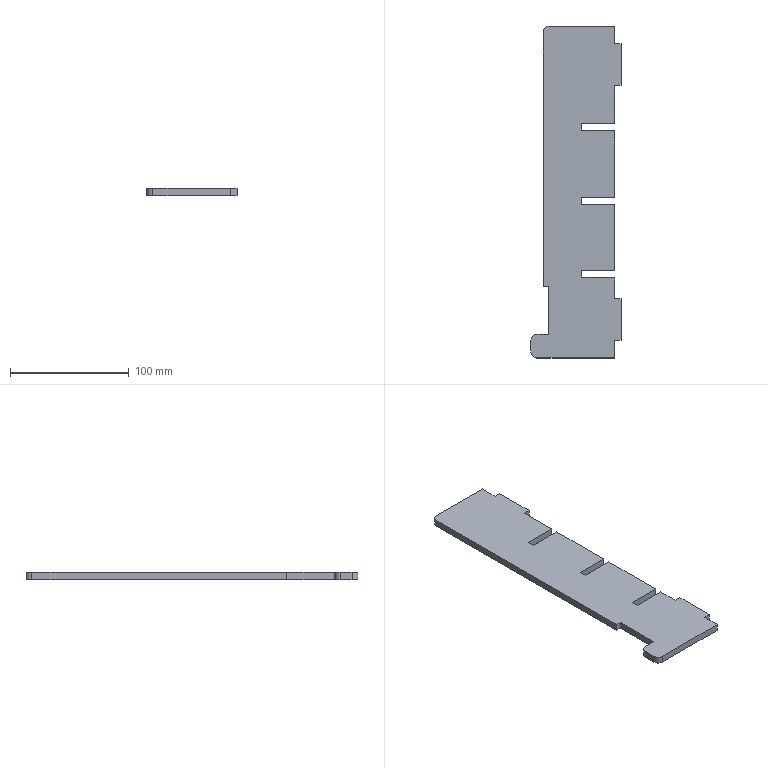Part | SolidWorks | features Fillet 1, FlatPattern 1, SMBaseFlange 1, SheetMetal 1 | 1 solid | 33 faces | box 76 x 280 x 6 mm | volume 100169 mm3 | plane 30 | cylinder 3 | commonest cylinder face diameters 10 x3
STEP:
#1=CARTESIAN_POINT('',(-245.,-135.834,0.));
#2=VERTEX_POINT('',#1);
#3=CARTESIAN_POINT('',(-255.,-135.834,0.));
#4=VERTEX_POINT('',#3);
#5=CARTESIAN_POINT('',(-245.,-135.834,0.));
#6=DIRECTION('',(-1.,0.,0.));
#7=VECTOR('',#6,1000.);
#8=LINE('',#5,#7);
#9=EDGE_CURVE('',#2,#4,#8,.T.);
#10=ORIENTED_EDGE('',*,*,#9,.T.);
#11=CARTESIAN_POINT('',(-255.,-135.834,6.));
#12=VERTEX_POINT('',#11);
#13=CARTESIAN_POINT('',(-255.,-135.834,6.));
#14=DIRECTION('',(0.,0.,1.));
#15=VECTOR('',#14,1000.);
#16=LINE('',#13,#15);
#17=EDGE_CURVE('',#4,#12,#16,.T.);
#18=ORIENTED_EDGE('',*,*,#17,.T.);
#19=CARTESIAN_POINT('',(-245.,-135.834,6.));
#20=VERTEX_POINT('',#19);
#21=CARTESIAN_POINT('',(-245.,-135.834,6.));
#22=DIRECTION('',(-1.,0.,0.));
#23=VECTOR('',#22,1000.);
#24=LINE('',#21,#23);
#25=EDGE_CURVE('',#20,#12,#24,.T.);
#26=ORIENTED_EDGE('',*,*,#25,.F.);
#27=CARTESIAN_POINT('',(-245.,-135.834,6.));
#28=DIRECTION('',(0.,0.,-1.));
#29=VECTOR('',#28,1000.);
#30=LINE('',#27,#29);
#31=EDGE_CURVE('',#20,#2,#30,.T.);
#32=ORIENTED_EDGE('',*,*,#31,.T.);
#33=EDGE_LOOP('',(#10,#18,#26,#32));
#34=FACE_OUTER_BOUND('',#33,.T.);
#35=CARTESIAN_POINT('',(-245.,-135.834,6.));
#36=DIRECTION('',(0.,-1.,0.));
#37=DIRECTION('',(0.,0.,-1.));
#38=AXIS2_PLACEMENT_3D('',#35,#36,#37);
#39=PLANE('',#38);
#40=ADVANCED_FACE('',(#34),#39,.F.);
#41=CARTESIAN_POINT('',(-260.,-140.834,6.));
#42=VERTEX_POINT('',#41);
#43=CARTESIAN_POINT('',(-260.,-150.834,6.));
#44=VERTEX_POINT('',#43);
#45=CARTESIAN_POINT('',(-260.,-135.834,6.));
#46=DIRECTION('',(0.,-1.,0.));
#47=VECTOR('',#46,1000.);
#48=LINE('',#45,#47);
#49=EDGE_CURVE('',#42,#44,#48,.T.);
#50=ORIENTED_EDGE('',*,*,#49,.F.);
#51=CARTESIAN_POINT('',(-260.,-140.834,0.));
#52=VERTEX_POINT('',#51);
#53=CARTESIAN_POINT('',(-260.,-140.834,6.));
#54=DIRECTION('',(0.,0.,-1.));
#55=VECTOR('',#54,1000.);
#56=LINE('',#53,#55);
#57=EDGE_CURVE('',#42,#52,#56,.T.);
#58=ORIENTED_EDGE('',*,*,#57,.T.);
#59=CARTESIAN_POINT('',(-260.,-150.834,0.));
#60=VERTEX_POINT('',#59);
#61=CARTESIAN_POINT('',(-260.,-135.834,0.));
#62=DIRECTION('',(0.,-1.,0.));
#63=VECTOR('',#62,1000.);
#64=LINE('',#61,#63);
#65=EDGE_CURVE('',#52,#60,#64,.T.);
#66=ORIENTED_EDGE('',*,*,#65,.T.);
#67=CARTESIAN_POINT('',(-260.,-150.834,6.));
#68=DIRECTION('',(0.,0.,1.));
#69=VECTOR('',#68,1000.);
#70=LINE('',#67,#69);
#71=EDGE_CURVE('',#60,#44,#70,.T.);
#72=ORIENTED_EDGE('',*,*,#71,.T.);
#73=EDGE_LOOP('',(#50,#58,#66,#72));
#74=FACE_OUTER_BOUND('',#73,.T.);
#75=CARTESIAN_POINT('',(-260.,-135.834,6.));
#76=DIRECTION('',(1.,0.,0.));
#77=DIRECTION('',(0.,0.,-1.));
#78=AXIS2_PLACEMENT_3D('',#75,#76,#77);
#79=PLANE('',#78);
#80=ADVANCED_FACE('',(#74),#79,.F.);
#81=CARTESIAN_POINT('',(-255.,-155.834,6.));
#82=VERTEX_POINT('',#81);
#83=CARTESIAN_POINT('',(-189.5,-155.834,6.));
#84=VERTEX_POINT('',#83);
#85=CARTESIAN_POINT('',(-260.,-155.834,6.));
#86=DIRECTION('',(1.,0.,0.));
#87=VECTOR('',#86,1000.);
#88=LINE('',#85,#87);
#89=EDGE_CURVE('',#82,#84,#88,.T.);
#90=ORIENTED_EDGE('',*,*,#89,.F.);
#91=CARTESIAN_POINT('',(-255.,-155.834,0.));
#92=VERTEX_POINT('',#91);
#93=CARTESIAN_POINT('',(-255.,-155.834,6.));
#94=DIRECTION('',(0.,0.,-1.));
#95=VECTOR('',#94,1000.);
#96=LINE('',#93,#95);
#97=EDGE_CURVE('',#82,#92,#96,.T.);
#98=ORIENTED_EDGE('',*,*,#97,.T.);
#99=CARTESIAN_POINT('',(-189.5,-155.834,0.));
#100=VERTEX_POINT('',#99);
#101=CARTESIAN_POINT('',(-260.,-155.834,0.));
#102=DIRECTION('',(1.,0.,0.));
#103=VECTOR('',#102,1000.);
#104=LINE('',#101,#103);
#105=EDGE_CURVE('',#92,#100,#104,.T.);
#106=ORIENTED_EDGE('',*,*,#105,.T.);
#107=CARTESIAN_POINT('',(-189.5,-155.834,6.));
#108=DIRECTION('',(0.,0.,-1.));
#109=VECTOR('',#108,1000.);
#110=LINE('',#107,#109);
#111=EDGE_CURVE('',#84,#100,#110,.T.);
#112=ORIENTED_EDGE('',*,*,#111,.F.);
#113=EDGE_LOOP('',(#90,#98,#106,#112));
#114=FACE_OUTER_BOUND('',#113,.T.);
#115=CARTESIAN_POINT('',(-260.,-155.834,6.));
#116=DIRECTION('',(0.,1.,0.));
#117=DIRECTION('',(0.,0.,1.));
#118=AXIS2_PLACEMENT_3D('',#115,#116,#117);
#119=PLANE('',#118);
#120=ADVANCED_FACE('',(#114),#119,.F.);
#121=CARTESIAN_POINT('',(-189.5,-140.834,0.));
#122=VERTEX_POINT('',#121);
#123=CARTESIAN_POINT('',(-189.5,-155.834,0.));
#124=DIRECTION('',(0.,1.,0.));
#125=VECTOR('',#124,1000.);
#126=LINE('',#123,#125);
#127=EDGE_CURVE('',#100,#122,#126,.T.);
#128=ORIENTED_EDGE('',*,*,#127,.T.);
#129=CARTESIAN_POINT('',(-189.5,-140.834,6.));
#130=VERTEX_POINT('',#129);
#131=CARTESIAN_POINT('',(-189.5,-140.834,6.));
#132=DIRECTION('',(0.,0.,-1.));
#133=VECTOR('',#132,1000.);
#134=LINE('',#131,#133);
#135=EDGE_CURVE('',#130,#122,#134,.T.);
#136=ORIENTED_EDGE('',*,*,#135,.F.);
#137=CARTESIAN_POINT('',(-189.5,-155.834,6.));
#138=DIRECTION('',(0.,1.,0.));
#139=VECTOR('',#138,1000.);
#140=LINE('',#137,#139);
#141=EDGE_CURVE('',#84,#130,#140,.T.);
#142=ORIENTED_EDGE('',*,*,#141,.F.);
#143=ORIENTED_EDGE('',*,*,#111,.T.);
#144=EDGE_LOOP('',(#128,#136,#142,#143));
#145=FACE_OUTER_BOUND('',#144,.T.);
#146=CARTESIAN_POINT('',(-189.5,-155.834,6.));
#147=DIRECTION('',(-1.,0.,0.));
#148=DIRECTION('',(0.,-1.,0.));
#149=AXIS2_PLACEMENT_3D('',#146,#147,#148);
#150=PLANE('',#149);
#151=ADVANCED_FACE('',(#145),#150,.F.);
#152=CARTESIAN_POINT('',(-184.,-140.834,0.));
#153=VERTEX_POINT('',#152);
#154=CARTESIAN_POINT('',(-189.5,-140.834,0.));
#155=DIRECTION('',(1.,0.,0.));
#156=VECTOR('',#155,1000.);
#157=LINE('',#154,#156);
#158=EDGE_CURVE('',#122,#153,#157,.T.);
#159=ORIENTED_EDGE('',*,*,#158,.T.);
#160=CARTESIAN_POINT('',(-184.,-140.834,6.));
#161=VERTEX_POINT('',#160);
#162=CARTESIAN_POINT('',(-184.,-140.834,6.));
#163=DIRECTION('',(0.,0.,-1.));
#164=VECTOR('',#163,1000.);
#165=LINE('',#162,#164);
#166=EDGE_CURVE('',#161,#153,#165,.T.);
#167=ORIENTED_EDGE('',*,*,#166,.F.);
#168=CARTESIAN_POINT('',(-189.5,-140.834,6.));
#169=DIRECTION('',(1.,0.,0.));
#170=VECTOR('',#169,1000.);
#171=LINE('',#168,#170);
#172=EDGE_CURVE('',#130,#161,#171,.T.);
#173=ORIENTED_EDGE('',*,*,#172,.F.);
#174=ORIENTED_EDGE('',*,*,#135,.T.);
#175=EDGE_LOOP('',(#159,#167,#173,#174));
#176=FACE_OUTER_BOUND('',#175,.T.);
#177=CARTESIAN_POINT('',(-189.5,-140.834,6.));
#178=DIRECTION('',(0.,1.,0.));
#179=DIRECTION('',(0.,0.,1.));
#180=AXIS2_PLACEMENT_3D('',#177,#178,#179);
#181=PLANE('',#180);
#182=ADVANCED_FACE('',(#176),#181,.F.);
#183=CARTESIAN_POINT('',(-184.,-105.834,0.));
#184=VERTEX_POINT('',#183);
#185=CARTESIAN_POINT('',(-184.,-140.834,0.));
#186=DIRECTION('',(0.,1.,0.));
#187=VECTOR('',#186,1000.);
#188=LINE('',#185,#187);
#189=EDGE_CURVE('',#153,#184,#188,.T.);
#190=ORIENTED_EDGE('',*,*,#189,.T.);
#191=CARTESIAN_POINT('',(-184.,-105.834,6.));
#192=VERTEX_POINT('',#191);
#193=CARTESIAN_POINT('',(-184.,-105.834,6.));
#194=DIRECTION('',(0.,0.,-1.));
#195=VECTOR('',#194,1000.);
#196=LINE('',#193,#195);
#197=EDGE_CURVE('',#192,#184,#196,.T.);
#198=ORIENTED_EDGE('',*,*,#197,.F.);
#199=CARTESIAN_POINT('',(-184.,-140.834,6.));
#200=DIRECTION('',(0.,1.,0.));
#201=VECTOR('',#200,1000.);
#202=LINE('',#199,#201);
#203=EDGE_CURVE('',#161,#192,#202,.T.);
#204=ORIENTED_EDGE('',*,*,#203,.F.);
#205=ORIENTED_EDGE('',*,*,#166,.T.);
#206=EDGE_LOOP('',(#190,#198,#204,#205));
#207=FACE_OUTER_BOUND('',#206,.T.);
#208=CARTESIAN_POINT('',(-184.,-140.834,6.));
#209=DIRECTION('',(-1.,0.,0.));
#210=DIRECTION('',(0.,0.,1.));
#211=AXIS2_PLACEMENT_3D('',#208,#209,#210);
#212=PLANE('',#211);
#213=ADVANCED_FACE('',(#207),#212,.F.);
#214=CARTESIAN_POINT('',(-189.5,-105.834,0.));
#215=VERTEX_POINT('',#214);
#216=CARTESIAN_POINT('',(-184.,-105.834,0.));
#217=DIRECTION('',(-1.,0.,0.));
#218=VECTOR('',#217,1000.);
#219=LINE('',#216,#218);
#220=EDGE_CURVE('',#184,#215,#219,.T.);
#221=ORIENTED_EDGE('',*,*,#220,.T.);
#222=CARTESIAN_POINT('',(-189.5,-105.834,6.));
#223=VERTEX_POINT('',#222);
#224=CARTESIAN_POINT('',(-189.5,-105.834,6.));
#225=DIRECTION('',(0.,0.,-1.));
#226=VECTOR('',#225,1000.);
#227=LINE('',#224,#226);
#228=EDGE_CURVE('',#223,#215,#227,.T.);
#229=ORIENTED_EDGE('',*,*,#228,.F.);
#230=CARTESIAN_POINT('',(-184.,-105.834,6.));
#231=DIRECTION('',(-1.,0.,0.));
#232=VECTOR('',#231,1000.);
#233=LINE('',#230,#232);
#234=EDGE_CURVE('',#192,#223,#233,.T.);
#235=ORIENTED_EDGE('',*,*,#234,.F.);
#236=ORIENTED_EDGE('',*,*,#197,.T.);
#237=EDGE_LOOP('',(#221,#229,#235,#236));
#238=FACE_OUTER_BOUND('',#237,.T.);
#239=CARTESIAN_POINT('',(-184.,-105.834,6.));
#240=DIRECTION('',(0.,-1.,0.));
#241=DIRECTION('',(0.,0.,-1.));
#242=AXIS2_PLACEMENT_3D('',#239,#240,#241);
#243=PLANE('',#242);
#244=ADVANCED_FACE('',(#238),#243,.F.);
#245=CARTESIAN_POINT('',(-189.5,-88.334,0.));
#246=VERTEX_POINT('',#245);
#247=CARTESIAN_POINT('',(-189.5,-105.834,0.));
#248=DIRECTION('',(0.,1.,0.));
#249=VECTOR('',#248,1000.);
#250=LINE('',#247,#249);
#251=EDGE_CURVE('',#215,#246,#250,.T.);
#252=ORIENTED_EDGE('',*,*,#251,.T.);
#253=CARTESIAN_POINT('',(-189.5,-88.334,6.));
#254=VERTEX_POINT('',#253);
#255=CARTESIAN_POINT('',(-189.5,-88.334,6.));
#256=DIRECTION('',(0.,0.,-1.));
#257=VECTOR('',#256,1000.);
#258=LINE('',#255,#257);
#259=EDGE_CURVE('',#254,#246,#258,.T.);
#260=ORIENTED_EDGE('',*,*,#259,.F.);
#261=CARTESIAN_POINT('',(-189.5,-105.834,6.));
#262=DIRECTION('',(0.,1.,0.));
#263=VECTOR('',#262,1000.);
#264=LINE('',#261,#263);
#265=EDGE_CURVE('',#223,#254,#264,.T.);
#266=ORIENTED_EDGE('',*,*,#265,.F.);
#267=ORIENTED_EDGE('',*,*,#228,.T.);
#268=EDGE_LOOP('',(#252,#260,#266,#267));
#269=FACE_OUTER_BOUND('',#268,.T.);
#270=CARTESIAN_POINT('',(-189.5,-105.834,6.));
#271=DIRECTION('',(-1.,0.,0.));
#272=DIRECTION('',(0.,0.,1.));
#273=AXIS2_PLACEMENT_3D('',#270,#271,#272);
#274=PLANE('',#273);
#275=ADVANCED_FACE('',(#269),#274,.F.);
#276=CARTESIAN_POINT('',(-217.5,-88.334,0.));
#277=VERTEX_POINT('',#276);
#278=CARTESIAN_POINT('',(-217.5,-88.334,0.));
#279=DIRECTION('',(-1.,0.,0.));
#280=VECTOR('',#279,1000.);
#281=LINE('',#278,#280);
#282=EDGE_CURVE('',#246,#277,#281,.T.);
#283=ORIENTED_EDGE('',*,*,#282,.T.);
#284=CARTESIAN_POINT('',(-217.5,-88.334,6.));
#285=VERTEX_POINT('',#284);
#286=CARTESIAN_POINT('',(-217.5,-88.334,6.));
#287=DIRECTION('',(0.,0.,-1.));
#288=VECTOR('',#287,1000.);
#289=LINE('',#286,#288);
#290=EDGE_CURVE('',#285,#277,#289,.T.);
#291=ORIENTED_EDGE('',*,*,#290,.F.);
#292=CARTESIAN_POINT('',(-217.5,-88.334,6.));
#293=DIRECTION('',(-1.,0.,0.));
#294=VECTOR('',#293,1000.);
#295=LINE('',#292,#294);
#296=EDGE_CURVE('',#254,#285,#295,.T.);
#297=ORIENTED_EDGE('',*,*,#296,.F.);
#298=ORIENTED_EDGE('',*,*,#259,.T.);
#299=EDGE_LOOP('',(#283,#291,#297,#298));
#300=FACE_OUTER_BOUND('',#299,.T.);
#301=CARTESIAN_POINT('',(-217.5,-88.334,6.));
#302=DIRECTION('',(0.,-1.,0.));
#303=DIRECTION('',(0.,0.,-1.));
#304=AXIS2_PLACEMENT_3D('',#301,#302,#303);
#305=PLANE('',#304);
#306=ADVANCED_FACE('',(#300),#305,.F.);
#307=CARTESIAN_POINT('',(-217.5,-82.334,0.));
#308=VERTEX_POINT('',#307);
#309=CARTESIAN_POINT('',(-217.5,-82.334,0.));
#310=DIRECTION('',(0.,1.,0.));
#311=VECTOR('',#310,1000.);
#312=LINE('',#309,#311);
#313=EDGE_CURVE('',#277,#308,#312,.T.);
#314=ORIENTED_EDGE('',*,*,#313,.T.);
#315=CARTESIAN_POINT('',(-217.5,-82.334,6.));
#316=VERTEX_POINT('',#315);
#317=CARTESIAN_POINT('',(-217.5,-82.334,6.));
#318=DIRECTION('',(0.,0.,-1.));
#319=VECTOR('',#318,1000.);
#320=LINE('',#317,#319);
#321=EDGE_CURVE('',#316,#308,#320,.T.);
#322=ORIENTED_EDGE('',*,*,#321,.F.);
#323=CARTESIAN_POINT('',(-217.5,-82.334,6.));
#324=DIRECTION('',(0.,1.,0.));
#325=VECTOR('',#324,1000.);
#326=LINE('',#323,#325);
#327=EDGE_CURVE('',#285,#316,#326,.T.);
#328=ORIENTED_EDGE('',*,*,#327,.F.);
#329=ORIENTED_EDGE('',*,*,#290,.T.);
#330=EDGE_LOOP('',(#314,#322,#328,#329));
#331=FACE_OUTER_BOUND('',#330,.T.);
#332=CARTESIAN_POINT('',(-217.5,-82.334,6.));
#333=DIRECTION('',(-1.,0.,0.));
#334=DIRECTION('',(0.,0.,1.));
#335=AXIS2_PLACEMENT_3D('',#332,#333,#334);
#336=PLANE('',#335);
#337=ADVANCED_FACE('',(#331),#336,.F.);
#338=CARTESIAN_POINT('',(-189.5,-82.334,0.));
#339=VERTEX_POINT('',#338);
#340=CARTESIAN_POINT('',(-189.5,-82.334,0.));
#341=DIRECTION('',(1.,0.,0.));
#342=VECTOR('',#341,1000.);
#343=LINE('',#340,#342);
#344=EDGE_CURVE('',#308,#339,#343,.T.);
#345=ORIENTED_EDGE('',*,*,#344,.T.);
#346=CARTESIAN_POINT('',(-189.5,-82.334,6.));
#347=VERTEX_POINT('',#346);
#348=CARTESIAN_POINT('',(-189.5,-82.334,6.));
#349=DIRECTION('',(0.,0.,-1.));
#350=VECTOR('',#349,1000.);
#351=LINE('',#348,#350);
#352=EDGE_CURVE('',#347,#339,#351,.T.);
#353=ORIENTED_EDGE('',*,*,#352,.F.);
#354=CARTESIAN_POINT('',(-189.5,-82.334,6.));
#355=DIRECTION('',(1.,0.,0.));
#356=VECTOR('',#355,1000.);
#357=LINE('',#354,#356);
#358=EDGE_CURVE('',#316,#347,#357,.T.);
#359=ORIENTED_EDGE('',*,*,#358,.F.);
#360=ORIENTED_EDGE('',*,*,#321,.T.);
#361=EDGE_LOOP('',(#345,#353,#359,#360));
#362=FACE_OUTER_BOUND('',#361,.T.);
#363=CARTESIAN_POINT('',(-189.5,-82.334,6.));
#364=DIRECTION('',(0.,1.,0.));
#365=DIRECTION('',(-1.,0.,0.));
#366=AXIS2_PLACEMENT_3D('',#363,#364,#365);
#367=PLANE('',#366);
#368=ADVANCED_FACE('',(#362),#367,.F.);
#369=CARTESIAN_POINT('',(-189.5,-26.334,0.));
#370=VERTEX_POINT('',#369);
#371=CARTESIAN_POINT('',(-189.5,-82.334,0.));
#372=DIRECTION('',(0.,1.,0.));
#373=VECTOR('',#372,1000.);
#374=LINE('',#371,#373);
#375=EDGE_CURVE('',#339,#370,#374,.T.);
#376=ORIENTED_EDGE('',*,*,#375,.T.);
#377=CARTESIAN_POINT('',(-189.5,-26.334,6.));
#378=VERTEX_POINT('',#377);
#379=CARTESIAN_POINT('',(-189.5,-26.334,6.));
#380=DIRECTION('',(0.,0.,-1.));
#381=VECTOR('',#380,1000.);
#382=LINE('',#379,#381);
#383=EDGE_CURVE('',#378,#370,#382,.T.);
#384=ORIENTED_EDGE('',*,*,#383,.F.);
#385=CARTESIAN_POINT('',(-189.5,-82.334,6.));
#386=DIRECTION('',(0.,1.,0.));
#387=VECTOR('',#386,1000.);
#388=LINE('',#385,#387);
#389=EDGE_CURVE('',#347,#378,#388,.T.);
#390=ORIENTED_EDGE('',*,*,#389,.F.);
#391=ORIENTED_EDGE('',*,*,#352,.T.);
#392=EDGE_LOOP('',(#376,#384,#390,#391));
#393=FACE_OUTER_BOUND('',#392,.T.);
#394=CARTESIAN_POINT('',(-189.5,-82.334,6.));
#395=DIRECTION('',(-1.,0.,0.));
#396=DIRECTION('',(0.,0.,1.));
#397=AXIS2_PLACEMENT_3D('',#394,#395,#396);
#398=PLANE('',#397);
#399=ADVANCED_FACE('',(#393),#398,.F.);
#400=CARTESIAN_POINT('',(-217.5,-26.334,0.));
#401=VERTEX_POINT('',#400);
#402=CARTESIAN_POINT('',(-217.5,-26.334,0.));
#403=DIRECTION('',(-1.,0.,0.));
#404=VECTOR('',#403,1000.);
#405=LINE('',#402,#404);
#406=EDGE_CURVE('',#370,#401,#405,.T.);
#407=ORIENTED_EDGE('',*,*,#406,.T.);
#408=CARTESIAN_POINT('',(-217.5,-26.334,6.));
#409=VERTEX_POINT('',#408);
#410=CARTESIAN_POINT('',(-217.5,-26.334,6.));
#411=DIRECTION('',(0.,0.,-1.));
#412=VECTOR('',#411,1000.);
#413=LINE('',#410,#412);
#414=EDGE_CURVE('',#409,#401,#413,.T.);
#415=ORIENTED_EDGE('',*,*,#414,.F.);
#416=CARTESIAN_POINT('',(-217.5,-26.334,6.));
#417=DIRECTION('',(-1.,0.,0.));
#418=VECTOR('',#417,1000.);
#419=LINE('',#416,#418);
#420=EDGE_CURVE('',#378,#409,#419,.T.);
#421=ORIENTED_EDGE('',*,*,#420,.F.);
#422=ORIENTED_EDGE('',*,*,#383,.T.);
#423=EDGE_LOOP('',(#407,#415,#421,#422));
#424=FACE_OUTER_BOUND('',#423,.T.);
#425=CARTESIAN_POINT('',(-217.5,-26.334,6.));
#426=DIRECTION('',(0.,-1.,0.));
#427=DIRECTION('',(0.,0.,-1.));
#428=AXIS2_PLACEMENT_3D('',#425,#426,#427);
#429=PLANE('',#428);
#430=ADVANCED_FACE('',(#424),#429,.F.);
#431=CARTESIAN_POINT('',(-217.5,-20.334,0.));
#432=VERTEX_POINT('',#431);
#433=CARTESIAN_POINT('',(-217.5,-20.334,0.));
#434=DIRECTION('',(0.,1.,0.));
#435=VECTOR('',#434,1000.);
#436=LINE('',#433,#435);
#437=EDGE_CURVE('',#401,#432,#436,.T.);
#438=ORIENTED_EDGE('',*,*,#437,.T.);
#439=CARTESIAN_POINT('',(-217.5,-20.334,6.));
#440=VERTEX_POINT('',#439);
#441=CARTESIAN_POINT('',(-217.5,-20.334,6.));
#442=DIRECTION('',(0.,0.,-1.));
#443=VECTOR('',#442,1000.);
#444=LINE('',#441,#443);
#445=EDGE_CURVE('',#440,#432,#444,.T.);
#446=ORIENTED_EDGE('',*,*,#445,.F.);
#447=CARTESIAN_POINT('',(-217.5,-20.334,6.));
#448=DIRECTION('',(0.,1.,0.));
#449=VECTOR('',#448,1000.);
#450=LINE('',#447,#449);
#451=EDGE_CURVE('',#409,#440,#450,.T.);
#452=ORIENTED_EDGE('',*,*,#451,.F.);
#453=ORIENTED_EDGE('',*,*,#414,.T.);
#454=EDGE_LOOP('',(#438,#446,#452,#453));
#455=FACE_OUTER_BOUND('',#454,.T.);
#456=CARTESIAN_POINT('',(-217.5,-20.334,6.));
#457=DIRECTION('',(-1.,0.,0.));
#458=DIRECTION('',(0.,0.,1.));
#459=AXIS2_PLACEMENT_3D('',#456,#457,#458);
#460=PLANE('',#459);
#461=ADVANCED_FACE('',(#455),#460,.F.);
#462=CARTESIAN_POINT('',(-189.5,-20.334,0.));
#463=VERTEX_POINT('',#462);
#464=CARTESIAN_POINT('',(-189.5,-20.334,0.));
#465=DIRECTION('',(1.,0.,0.));
#466=VECTOR('',#465,1000.);
#467=LINE('',#464,#466);
#468=EDGE_CURVE('',#432,#463,#467,.T.);
#469=ORIENTED_EDGE('',*,*,#468,.T.);
#470=CARTESIAN_POINT('',(-189.5,-20.334,6.));
#471=VERTEX_POINT('',#470);
#472=CARTESIAN_POINT('',(-189.5,-20.334,6.));
#473=DIRECTION('',(0.,0.,-1.));
#474=VECTOR('',#473,1000.);
#475=LINE('',#472,#474);
#476=EDGE_CURVE('',#471,#463,#475,.T.);
#477=ORIENTED_EDGE('',*,*,#476,.F.);
#478=CARTESIAN_POINT('',(-189.5,-20.334,6.));
#479=DIRECTION('',(1.,0.,0.));
#480=VECTOR('',#479,1000.);
#481=LINE('',#478,#480);
#482=EDGE_CURVE('',#440,#471,#481,.T.);
#483=ORIENTED_EDGE('',*,*,#482,.F.);
#484=ORIENTED_EDGE('',*,*,#445,.T.);
#485=EDGE_LOOP('',(#469,#477,#483,#484));
#486=FACE_OUTER_BOUND('',#485,.T.);
#487=CARTESIAN_POINT('',(-189.5,-20.334,6.));
#488=DIRECTION('',(0.,1.,0.));
#489=DIRECTION('',(0.,0.,1.));
#490=AXIS2_PLACEMENT_3D('',#487,#488,#489);
#491=PLANE('',#490);
#492=ADVANCED_FACE('',(#486),#491,.F.);
#493=CARTESIAN_POINT('',(-189.5,35.666,0.));
#494=VERTEX_POINT('',#493);
#495=CARTESIAN_POINT('',(-189.5,-20.334,0.));
#496=DIRECTION('',(0.,1.,0.));
#497=VECTOR('',#496,1000.);
#498=LINE('',#495,#497);
#499=EDGE_CURVE('',#463,#494,#498,.T.);
#500=ORIENTED_EDGE('',*,*,#499,.T.);
#501=CARTESIAN_POINT('',(-189.5,35.666,6.));
#502=VERTEX_POINT('',#501);
#503=CARTESIAN_POINT('',(-189.5,35.666,6.));
#504=DIRECTION('',(0.,0.,-1.));
#505=VECTOR('',#504,1000.);
#506=LINE('',#503,#505);
#507=EDGE_CURVE('',#502,#494,#506,.T.);
#508=ORIENTED_EDGE('',*,*,#507,.F.);
#509=CARTESIAN_POINT('',(-189.5,-20.334,6.));
#510=DIRECTION('',(0.,1.,0.));
#511=VECTOR('',#510,1000.);
#512=LINE('',#509,#511);
#513=EDGE_CURVE('',#471,#502,#512,.T.);
#514=ORIENTED_EDGE('',*,*,#513,.F.);
#515=ORIENTED_EDGE('',*,*,#476,.T.);
#516=EDGE_LOOP('',(#500,#508,#514,#515));
#517=FACE_OUTER_BOUND('',#516,.T.);
#518=CARTESIAN_POINT('',(-189.5,-20.334,6.));
#519=DIRECTION('',(-1.,0.,0.));
#520=DIRECTION('',(0.,0.,1.));
#521=AXIS2_PLACEMENT_3D('',#518,#519,#520);
#522=PLANE('',#521);
#523=ADVANCED_FACE('',(#517),#522,.F.);
#524=CARTESIAN_POINT('',(-217.5,35.666,0.));
#525=VERTEX_POINT('',#524);
#526=CARTESIAN_POINT('',(-217.5,35.666,0.));
#527=DIRECTION('',(-1.,0.,0.));
#528=VECTOR('',#527,1000.);
#529=LINE('',#526,#528);
#530=EDGE_CURVE('',#494,#525,#529,.T.);
#531=ORIENTED_EDGE('',*,*,#530,.T.);
#532=CARTESIAN_POINT('',(-217.5,35.666,6.));
#533=VERTEX_POINT('',#532);
#534=CARTESIAN_POINT('',(-217.5,35.666,6.));
#535=DIRECTION('',(0.,0.,-1.));
#536=VECTOR('',#535,1000.);
#537=LINE('',#534,#536);
#538=EDGE_CURVE('',#533,#525,#537,.T.);
#539=ORIENTED_EDGE('',*,*,#538,.F.);
#540=CARTESIAN_POINT('',(-217.5,35.666,6.));
#541=DIRECTION('',(-1.,0.,0.));
#542=VECTOR('',#541,1000.);
#543=LINE('',#540,#542);
#544=EDGE_CURVE('',#502,#533,#543,.T.);
#545=ORIENTED_EDGE('',*,*,#544,.F.);
#546=ORIENTED_EDGE('',*,*,#507,.T.);
#547=EDGE_LOOP('',(#531,#539,#545,#546));
#548=FACE_OUTER_BOUND('',#547,.T.);
#549=CARTESIAN_POINT('',(-217.5,35.666,6.));
#550=DIRECTION('',(0.,-1.,0.));
#551=DIRECTION('',(0.,0.,-1.));
#552=AXIS2_PLACEMENT_3D('',#549,#550,#551);
#553=PLANE('',#552);
#554=ADVANCED_FACE('',(#548),#553,.F.);
#555=CARTESIAN_POINT('',(-217.5,41.666,0.));
#556=VERTEX_POINT('',#555);
#557=CARTESIAN_POINT('',(-217.5,41.666,0.));
#558=DIRECTION('',(0.,1.,0.));
#559=VECTOR('',#558,1000.);
#560=LINE('',#557,#559);
#561=EDGE_CURVE('',#525,#556,#560,.T.);
#562=ORIENTED_EDGE('',*,*,#561,.T.);
#563=CARTESIAN_POINT('',(-217.5,41.666,6.));
#564=VERTEX_POINT('',#563);
#565=CARTESIAN_POINT('',(-217.5,41.666,6.));
#566=DIRECTION('',(0.,0.,-1.));
#567=VECTOR('',#566,1000.);
#568=LINE('',#565,#567);
#569=EDGE_CURVE('',#564,#556,#568,.T.);
#570=ORIENTED_EDGE('',*,*,#569,.F.);
#571=CARTESIAN_POINT('',(-217.5,41.666,6.));
#572=DIRECTION('',(0.,1.,0.));
#573=VECTOR('',#572,1000.);
#574=LINE('',#571,#573);
#575=EDGE_CURVE('',#533,#564,#574,.T.);
#576=ORIENTED_EDGE('',*,*,#575,.F.);
#577=ORIENTED_EDGE('',*,*,#538,.T.);
#578=EDGE_LOOP('',(#562,#570,#576,#577));
#579=FACE_OUTER_BOUND('',#578,.T.);
#580=CARTESIAN_POINT('',(-217.5,41.666,6.));
#581=DIRECTION('',(-1.,0.,0.));
#582=DIRECTION('',(0.,0.,1.));
#583=AXIS2_PLACEMENT_3D('',#580,#581,#582);
#584=PLANE('',#583);
#585=ADVANCED_FACE('',(#579),#584,.F.);
#586=CARTESIAN_POINT('',(-189.5,41.666,0.));
#587=VERTEX_POINT('',#586);
#588=CARTESIAN_POINT('',(-189.5,41.666,0.));
#589=DIRECTION('',(1.,0.,0.));
#590=VECTOR('',#589,1000.);
#591=LINE('',#588,#590);
#592=EDGE_CURVE('',#556,#587,#591,.T.);
#593=ORIENTED_EDGE('',*,*,#592,.T.);
#594=CARTESIAN_POINT('',(-189.5,41.666,6.));
#595=VERTEX_POINT('',#594);
#596=CARTESIAN_POINT('',(-189.5,41.666,6.));
#597=DIRECTION('',(0.,0.,-1.));
#598=VECTOR('',#597,1000.);
#599=LINE('',#596,#598);
#600=EDGE_CURVE('',#595,#587,#599,.T.);
#601=ORIENTED_EDGE('',*,*,#600,.F.);
#602=CARTESIAN_POINT('',(-189.5,41.666,6.));
#603=DIRECTION('',(1.,0.,0.));
#604=VECTOR('',#603,1000.);
#605=LINE('',#602,#604);
#606=EDGE_CURVE('',#564,#595,#605,.T.);
#607=ORIENTED_EDGE('',*,*,#606,.F.);
#608=ORIENTED_EDGE('',*,*,#569,.T.);
#609=EDGE_LOOP('',(#593,#601,#607,#608));
#610=FACE_OUTER_BOUND('',#609,.T.);
#611=CARTESIAN_POINT('',(-189.5,41.666,6.));
#612=DIRECTION('',(0.,1.,0.));
#613=DIRECTION('',(0.,0.,1.));
#614=AXIS2_PLACEMENT_3D('',#611,#612,#613);
#615=PLANE('',#614);
#616=ADVANCED_FACE('',(#610),#615,.F.);
#617=CARTESIAN_POINT('',(-189.5,74.166,0.));
#618=VERTEX_POINT('',#617);
#619=CARTESIAN_POINT('',(-189.5,41.666,0.));
#620=DIRECTION('',(0.,1.,0.));
#621=VECTOR('',#620,1000.);
#622=LINE('',#619,#621);
#623=EDGE_CURVE('',#587,#618,#622,.T.);
#624=ORIENTED_EDGE('',*,*,#623,.T.);
#625=CARTESIAN_POINT('',(-189.5,74.166,6.));
#626=VERTEX_POINT('',#625);
#627=CARTESIAN_POINT('',(-189.5,74.166,6.));
#628=DIRECTION('',(0.,0.,-1.));
#629=VECTOR('',#628,1000.);
#630=LINE('',#627,#629);
#631=EDGE_CURVE('',#626,#618,#630,.T.);
#632=ORIENTED_EDGE('',*,*,#631,.F.);
#633=CARTESIAN_POINT('',(-189.5,41.666,6.));
#634=DIRECTION('',(0.,1.,0.));
#635=VECTOR('',#634,1000.);
#636=LINE('',#633,#635);
#637=EDGE_CURVE('',#595,#626,#636,.T.);
#638=ORIENTED_EDGE('',*,*,#637,.F.);
#639=ORIENTED_EDGE('',*,*,#600,.T.);
#640=EDGE_LOOP('',(#624,#632,#638,#639));
#641=FACE_OUTER_BOUND('',#640,.T.);
#642=CARTESIAN_POINT('',(-189.5,41.666,6.));
#643=DIRECTION('',(-1.,0.,0.));
#644=DIRECTION('',(0.,0.,1.));
#645=AXIS2_PLACEMENT_3D('',#642,#643,#644);
#646=PLANE('',#645);
#647=ADVANCED_FACE('',(#641),#646,.F.);
#648=CARTESIAN_POINT('',(-184.,74.166,0.));
#649=VERTEX_POINT('',#648);
#650=CARTESIAN_POINT('',(-184.,74.166,0.));
#651=DIRECTION('',(1.,0.,0.));
#652=VECTOR('',#651,1000.);
#653=LINE('',#650,#652);
#654=EDGE_CURVE('',#618,#649,#653,.T.);
#655=ORIENTED_EDGE('',*,*,#654,.T.);
#656=CARTESIAN_POINT('',(-184.,74.166,6.));
#657=VERTEX_POINT('',#656);
#658=CARTESIAN_POINT('',(-184.,74.166,6.));
#659=DIRECTION('',(0.,0.,-1.));
#660=VECTOR('',#659,1000.);
#661=LINE('',#658,#660);
#662=EDGE_CURVE('',#657,#649,#661,.T.);
#663=ORIENTED_EDGE('',*,*,#662,.F.);
#664=CARTESIAN_POINT('',(-184.,74.166,6.));
#665=DIRECTION('',(1.,0.,0.));
#666=VECTOR('',#665,1000.);
#667=LINE('',#664,#666);
#668=EDGE_CURVE('',#626,#657,#667,.T.);
#669=ORIENTED_EDGE('',*,*,#668,.F.);
#670=ORIENTED_EDGE('',*,*,#631,.T.);
#671=EDGE_LOOP('',(#655,#663,#669,#670));
#672=FACE_OUTER_BOUND('',#671,.T.);
#673=CARTESIAN_POINT('',(-184.,74.166,6.));
#674=DIRECTION('',(0.,1.,0.));
#675=DIRECTION('',(0.,0.,1.));
#676=AXIS2_PLACEMENT_3D('',#673,#674,#675);
#677=PLANE('',#676);
#678=ADVANCED_FACE('',(#672),#677,.F.);
#679=CARTESIAN_POINT('',(-184.,109.166,0.));
#680=VERTEX_POINT('',#679);
#681=CARTESIAN_POINT('',(-184.,109.166,0.));
#682=DIRECTION('',(0.,1.,0.));
#683=VECTOR('',#682,1000.);
#684=LINE('',#681,#683);
#685=EDGE_CURVE('',#649,#680,#684,.T.);
#686=ORIENTED_EDGE('',*,*,#685,.T.);
#687=CARTESIAN_POINT('',(-184.,109.166,6.));
#688=VERTEX_POINT('',#687);
#689=CARTESIAN_POINT('',(-184.,109.166,6.));
#690=DIRECTION('',(0.,0.,-1.));
#691=VECTOR('',#690,1000.);
#692=LINE('',#689,#691);
#693=EDGE_CURVE('',#688,#680,#692,.T.);
#694=ORIENTED_EDGE('',*,*,#693,.F.);
#695=CARTESIAN_POINT('',(-184.,109.166,6.));
#696=DIRECTION('',(0.,1.,0.));
#697=VECTOR('',#696,1000.);
#698=LINE('',#695,#697);
#699=EDGE_CURVE('',#657,#688,#698,.T.);
#700=ORIENTED_EDGE('',*,*,#699,.F.);
#701=ORIENTED_EDGE('',*,*,#662,.T.);
#702=EDGE_LOOP('',(#686,#694,#700,#701));
#703=FACE_OUTER_BOUND('',#702,.T.);
#704=CARTESIAN_POINT('',(-184.,109.166,6.));
#705=DIRECTION('',(-1.,0.,0.));
#706=DIRECTION('',(0.,0.,1.));
#707=AXIS2_PLACEMENT_3D('',#704,#705,#706);
#708=PLANE('',#707);
#709=ADVANCED_FACE('',(#703),#708,.F.);
#710=CARTESIAN_POINT('',(-189.5,109.166,0.));
#711=VERTEX_POINT('',#710);
#712=CARTESIAN_POINT('',(-189.5,109.166,0.));
#713=DIRECTION('',(-1.,0.,0.));
#714=VECTOR('',#713,1000.);
#715=LINE('',#712,#714);
#716=EDGE_CURVE('',#680,#711,#715,.T.);
#717=ORIENTED_EDGE('',*,*,#716,.T.);
#718=CARTESIAN_POINT('',(-189.5,109.166,6.));
#719=VERTEX_POINT('',#718);
#720=CARTESIAN_POINT('',(-189.5,109.166,6.));
#721=DIRECTION('',(0.,0.,-1.));
#722=VECTOR('',#721,1000.);
#723=LINE('',#720,#722);
#724=EDGE_CURVE('',#719,#711,#723,.T.);
#725=ORIENTED_EDGE('',*,*,#724,.F.);
#726=CARTESIAN_POINT('',(-189.5,109.166,6.));
#727=DIRECTION('',(-1.,0.,0.));
#728=VECTOR('',#727,1000.);
#729=LINE('',#726,#728);
#730=EDGE_CURVE('',#688,#719,#729,.T.);
#731=ORIENTED_EDGE('',*,*,#730,.F.);
#732=ORIENTED_EDGE('',*,*,#693,.T.);
#733=EDGE_LOOP('',(#717,#725,#731,#732));
#734=FACE_OUTER_BOUND('',#733,.T.);
#735=CARTESIAN_POINT('',(-189.5,109.166,6.));
#736=DIRECTION('',(0.,-1.,0.));
#737=DIRECTION('',(0.,0.,-1.));
#738=AXIS2_PLACEMENT_3D('',#735,#736,#737);
#739=PLANE('',#738);
#740=ADVANCED_FACE('',(#734),#739,.F.);
#741=CARTESIAN_POINT('',(-189.5,124.166,0.));
#742=VERTEX_POINT('',#741);
#743=CARTESIAN_POINT('',(-189.5,109.166,0.));
#744=DIRECTION('',(0.,1.,0.));
#745=VECTOR('',#744,1000.);
#746=LINE('',#743,#745);
#747=EDGE_CURVE('',#711,#742,#746,.T.);
#748=ORIENTED_EDGE('',*,*,#747,.T.);
#749=CARTESIAN_POINT('',(-189.5,124.166,6.));
#750=VERTEX_POINT('',#749);
#751=CARTESIAN_POINT('',(-189.5,124.166,6.));
#752=DIRECTION('',(0.,0.,-1.));
#753=VECTOR('',#752,1000.);
#754=LINE('',#751,#753);
#755=EDGE_CURVE('',#750,#742,#754,.T.);
#756=ORIENTED_EDGE('',*,*,#755,.F.);
#757=CARTESIAN_POINT('',(-189.5,109.166,6.));
#758=DIRECTION('',(0.,1.,0.));
#759=VECTOR('',#758,1000.);
#760=LINE('',#757,#759);
#761=EDGE_CURVE('',#719,#750,#760,.T.);
#762=ORIENTED_EDGE('',*,*,#761,.F.);
#763=ORIENTED_EDGE('',*,*,#724,.T.);
#764=EDGE_LOOP('',(#748,#756,#762,#763));
#765=FACE_OUTER_BOUND('',#764,.T.);
#766=CARTESIAN_POINT('',(-189.5,109.166,6.));
#767=DIRECTION('',(-1.,0.,0.));
#768=DIRECTION('',(0.,-1.,0.));
#769=AXIS2_PLACEMENT_3D('',#766,#767,#768);
#770=PLANE('',#769);
#771=ADVANCED_FACE('',(#765),#770,.F.);
#772=CARTESIAN_POINT('',(-244.5,124.166,0.));
#773=VERTEX_POINT('',#772);
#774=CARTESIAN_POINT('',(-189.5,124.166,0.));
#775=DIRECTION('',(-1.,0.,0.));
#776=VECTOR('',#775,1000.);
#777=LINE('',#774,#776);
#778=EDGE_CURVE('',#742,#773,#777,.T.);
#779=ORIENTED_EDGE('',*,*,#778,.T.);
#780=CARTESIAN_POINT('',(-244.5,124.166,6.));
#781=VERTEX_POINT('',#780);
#782=CARTESIAN_POINT('',(-244.5,124.166,6.));
#783=DIRECTION('',(0.,0.,1.));
#784=VECTOR('',#783,1000.);
#785=LINE('',#782,#784);
#786=EDGE_CURVE('',#773,#781,#785,.T.);
#787=ORIENTED_EDGE('',*,*,#786,.T.);
#788=CARTESIAN_POINT('',(-189.5,124.166,6.));
#789=DIRECTION('',(-1.,0.,0.));
#790=VECTOR('',#789,1000.);
#791=LINE('',#788,#790);
#792=EDGE_CURVE('',#750,#781,#791,.T.);
#793=ORIENTED_EDGE('',*,*,#792,.F.);
#794=ORIENTED_EDGE('',*,*,#755,.T.);
#795=EDGE_LOOP('',(#779,#787,#793,#794));
#796=FACE_OUTER_BOUND('',#795,.T.);
#797=CARTESIAN_POINT('',(-189.5,124.166,6.));
#798=DIRECTION('',(0.,-1.,0.));
#799=DIRECTION('',(0.,0.,-1.));
#800=AXIS2_PLACEMENT_3D('',#797,#798,#799);
#801=PLANE('',#800);
#802=ADVANCED_FACE('',(#796),#801,.F.);
#803=CARTESIAN_POINT('',(-249.5,119.166,6.));
#804=VERTEX_POINT('',#803);
#805=CARTESIAN_POINT('',(-249.5,-95.834,6.));
#806=VERTEX_POINT('',#805);
#807=CARTESIAN_POINT('',(-249.5,124.166,6.));
#808=DIRECTION('',(0.,-1.,0.));
#809=VECTOR('',#808,1000.);
#810=LINE('',#807,#809);
#811=EDGE_CURVE('',#804,#806,#810,.T.);
#812=ORIENTED_EDGE('',*,*,#811,.F.);
#813=CARTESIAN_POINT('',(-249.5,119.166,0.));
#814=VERTEX_POINT('',#813);
#815=CARTESIAN_POINT('',(-249.5,119.166,6.));
#816=DIRECTION('',(0.,0.,-1.));
#817=VECTOR('',#816,1000.);
#818=LINE('',#815,#817);
#819=EDGE_CURVE('',#804,#814,#818,.T.);
#820=ORIENTED_EDGE('',*,*,#819,.T.);
#821=CARTESIAN_POINT('',(-249.5,-95.834,0.));
#822=VERTEX_POINT('',#821);
#823=CARTESIAN_POINT('',(-249.5,124.166,0.));
#824=DIRECTION('',(0.,-1.,0.));
#825=VECTOR('',#824,1000.);
#826=LINE('',#823,#825);
#827=EDGE_CURVE('',#814,#822,#826,.T.);
#828=ORIENTED_EDGE('',*,*,#827,.T.);
#829=CARTESIAN_POINT('',(-249.5,-95.834,6.));
#830=DIRECTION('',(0.,0.,-1.));
#831=VECTOR('',#830,1000.);
#832=LINE('',#829,#831);
#833=EDGE_CURVE('',#806,#822,#832,.T.);
#834=ORIENTED_EDGE('',*,*,#833,.F.);
#835=EDGE_LOOP('',(#812,#820,#828,#834));
#836=FACE_OUTER_BOUND('',#835,.T.);
#837=CARTESIAN_POINT('',(-249.5,124.166,6.));
#838=DIRECTION('',(1.,0.,0.));
#839=DIRECTION('',(0.,1.,0.));
#840=AXIS2_PLACEMENT_3D('',#837,#838,#839);
#841=PLANE('',#840);
#842=ADVANCED_FACE('',(#836),#841,.F.);
#843=CARTESIAN_POINT('',(-245.,-95.834,0.));
#844=VERTEX_POINT('',#843);
#845=CARTESIAN_POINT('',(-249.5,-95.834,0.));
#846=DIRECTION('',(1.,0.,0.));
#847=VECTOR('',#846,1000.);
#848=LINE('',#845,#847);
#849=EDGE_CURVE('',#822,#844,#848,.T.);
#850=ORIENTED_EDGE('',*,*,#849,.T.);
#851=CARTESIAN_POINT('',(-245.,-95.834,6.));
#852=VERTEX_POINT('',#851);
#853=CARTESIAN_POINT('',(-245.,-95.834,6.));
#854=DIRECTION('',(0.,0.,-1.));
#855=VECTOR('',#854,1000.);
#856=LINE('',#853,#855);
#857=EDGE_CURVE('',#852,#844,#856,.T.);
#858=ORIENTED_EDGE('',*,*,#857,.F.);
#859=CARTESIAN_POINT('',(-249.5,-95.834,6.));
#860=DIRECTION('',(1.,0.,0.));
#861=VECTOR('',#860,1000.);
#862=LINE('',#859,#861);
#863=EDGE_CURVE('',#806,#852,#862,.T.);
#864=ORIENTED_EDGE('',*,*,#863,.F.);
#865=ORIENTED_EDGE('',*,*,#833,.T.);
#866=EDGE_LOOP('',(#850,#858,#864,#865));
#867=FACE_OUTER_BOUND('',#866,.T.);
#868=CARTESIAN_POINT('',(-249.5,-95.834,6.));
#869=DIRECTION('',(0.,1.,0.));
#870=DIRECTION('',(0.,0.,1.));
#871=AXIS2_PLACEMENT_3D('',#868,#869,#870);
#872=PLANE('',#871);
#873=ADVANCED_FACE('',(#867),#872,.F.);
#874=CARTESIAN_POINT('',(-245.,-95.834,0.));
#875=DIRECTION('',(0.,-1.,0.));
#876=VECTOR('',#875,1000.);
#877=LINE('',#874,#876);
#878=EDGE_CURVE('',#844,#2,#877,.T.);
#879=ORIENTED_EDGE('',*,*,#878,.T.);
#880=ORIENTED_EDGE('',*,*,#31,.F.);
#881=CARTESIAN_POINT('',(-245.,-95.834,6.));
#882=DIRECTION('',(0.,-1.,0.));
#883=VECTOR('',#882,1000.);
#884=LINE('',#881,#883);
#885=EDGE_CURVE('',#852,#20,#884,.T.);
#886=ORIENTED_EDGE('',*,*,#885,.F.);
#887=ORIENTED_EDGE('',*,*,#857,.T.);
#888=EDGE_LOOP('',(#879,#880,#886,#887));
#889=FACE_OUTER_BOUND('',#888,.T.);
#890=CARTESIAN_POINT('',(-245.,-95.834,6.));
#891=DIRECTION('',(1.,0.,0.));
#892=DIRECTION('',(0.,0.,-1.));
#893=AXIS2_PLACEMENT_3D('',#890,#891,#892);
#894=PLANE('',#893);
#895=ADVANCED_FACE('',(#889),#894,.F.);
#896=ORIENTED_EDGE('',*,*,#25,.T.);
#897=CARTESIAN_POINT('',(-255.,-140.834,6.));
#898=DIRECTION('',(0.,0.,1.));
#899=DIRECTION('',(1.,0.,0.));
#900=AXIS2_PLACEMENT_3D('',#897,#898,#899);
#901=CIRCLE('',#900,5.);
#902=EDGE_CURVE('',#12,#42,#901,.T.);
#903=ORIENTED_EDGE('',*,*,#902,.T.);
#904=ORIENTED_EDGE('',*,*,#49,.T.);
#905=CARTESIAN_POINT('',(-255.,-150.834,6.));
#906=DIRECTION('',(0.,0.,1.));
#907=DIRECTION('',(1.,0.,0.));
#908=AXIS2_PLACEMENT_3D('',#905,#906,#907);
#909=CIRCLE('',#908,5.);
#910=EDGE_CURVE('',#44,#82,#909,.T.);
#911=ORIENTED_EDGE('',*,*,#910,.T.);
#912=ORIENTED_EDGE('',*,*,#89,.T.);
#913=ORIENTED_EDGE('',*,*,#141,.T.);
#914=ORIENTED_EDGE('',*,*,#172,.T.);
#915=ORIENTED_EDGE('',*,*,#203,.T.);
#916=ORIENTED_EDGE('',*,*,#234,.T.);
#917=ORIENTED_EDGE('',*,*,#265,.T.);
#918=ORIENTED_EDGE('',*,*,#296,.T.);
#919=ORIENTED_EDGE('',*,*,#327,.T.);
#920=ORIENTED_EDGE('',*,*,#358,.T.);
#921=ORIENTED_EDGE('',*,*,#389,.T.);
#922=ORIENTED_EDGE('',*,*,#420,.T.);
#923=ORIENTED_EDGE('',*,*,#451,.T.);
#924=ORIENTED_EDGE('',*,*,#482,.T.);
#925=ORIENTED_EDGE('',*,*,#513,.T.);
#926=ORIENTED_EDGE('',*,*,#544,.T.);
#927=ORIENTED_EDGE('',*,*,#575,.T.);
#928=ORIENTED_EDGE('',*,*,#606,.T.);
#929=ORIENTED_EDGE('',*,*,#637,.T.);
#930=ORIENTED_EDGE('',*,*,#668,.T.);
#931=ORIENTED_EDGE('',*,*,#699,.T.);
#932=ORIENTED_EDGE('',*,*,#730,.T.);
#933=ORIENTED_EDGE('',*,*,#761,.T.);
#934=ORIENTED_EDGE('',*,*,#792,.T.);
#935=CARTESIAN_POINT('',(-244.5,119.166,6.));
#936=DIRECTION('',(0.,0.,1.));
#937=DIRECTION('',(1.,0.,0.));
#938=AXIS2_PLACEMENT_3D('',#935,#936,#937);
#939=CIRCLE('',#938,5.);
#940=EDGE_CURVE('',#781,#804,#939,.T.);
#941=ORIENTED_EDGE('',*,*,#940,.T.);
#942=ORIENTED_EDGE('',*,*,#811,.T.);
#943=ORIENTED_EDGE('',*,*,#863,.T.);
#944=ORIENTED_EDGE('',*,*,#885,.T.);
#945=EDGE_LOOP('',(#896,#903,#904,#911,#912,#913,#914,#915,#916,#917,#918,#919,#920,#921,#922,#923,#924,#925,#926,#927,#928,#929,#930,#931,#932,#933,#934,#941,#942,#943,#944));
#946=FACE_OUTER_BOUND('',#945,.T.);
#947=CARTESIAN_POINT('',(0.,0.,6.));
#948=DIRECTION('',(0.,0.,1.));
#949=DIRECTION('',(1.,0.,0.));
#950=AXIS2_PLACEMENT_3D('',#947,#948,#949);
#951=PLANE('',#950);
#952=ADVANCED_FACE('',(#946),#951,.T.);
#953=ORIENTED_EDGE('',*,*,#65,.F.);
#954=CARTESIAN_POINT('',(-255.,-140.834,0.));
#955=DIRECTION('',(0.,0.,-1.));
#956=DIRECTION('',(1.,0.,0.));
#957=AXIS2_PLACEMENT_3D('',#954,#955,#956);
#958=CIRCLE('',#957,5.);
#959=EDGE_CURVE('',#52,#4,#958,.T.);
#960=ORIENTED_EDGE('',*,*,#959,.T.);
#961=ORIENTED_EDGE('',*,*,#9,.F.);
#962=ORIENTED_EDGE('',*,*,#878,.F.);
#963=ORIENTED_EDGE('',*,*,#849,.F.);
#964=ORIENTED_EDGE('',*,*,#827,.F.);
#965=CARTESIAN_POINT('',(-244.5,119.166,0.));
#966=DIRECTION('',(0.,0.,-1.));
#967=DIRECTION('',(1.,0.,0.));
#968=AXIS2_PLACEMENT_3D('',#965,#966,#967);
#969=CIRCLE('',#968,5.);
#970=EDGE_CURVE('',#814,#773,#969,.T.);
#971=ORIENTED_EDGE('',*,*,#970,.T.);
#972=ORIENTED_EDGE('',*,*,#778,.F.);
#973=ORIENTED_EDGE('',*,*,#747,.F.);
#974=ORIENTED_EDGE('',*,*,#716,.F.);
#975=ORIENTED_EDGE('',*,*,#685,.F.);
#976=ORIENTED_EDGE('',*,*,#654,.F.);
#977=ORIENTED_EDGE('',*,*,#623,.F.);
#978=ORIENTED_EDGE('',*,*,#592,.F.);
#979=ORIENTED_EDGE('',*,*,#561,.F.);
#980=ORIENTED_EDGE('',*,*,#530,.F.);
#981=ORIENTED_EDGE('',*,*,#499,.F.);
#982=ORIENTED_EDGE('',*,*,#468,.F.);
#983=ORIENTED_EDGE('',*,*,#437,.F.);
#984=ORIENTED_EDGE('',*,*,#406,.F.);
#985=ORIENTED_EDGE('',*,*,#375,.F.);
#986=ORIENTED_EDGE('',*,*,#344,.F.);
#987=ORIENTED_EDGE('',*,*,#313,.F.);
#988=ORIENTED_EDGE('',*,*,#282,.F.);
#989=ORIENTED_EDGE('',*,*,#251,.F.);
#990=ORIENTED_EDGE('',*,*,#220,.F.);
#991=ORIENTED_EDGE('',*,*,#189,.F.);
#992=ORIENTED_EDGE('',*,*,#158,.F.);
#993=ORIENTED_EDGE('',*,*,#127,.F.);
#994=ORIENTED_EDGE('',*,*,#105,.F.);
#995=CARTESIAN_POINT('',(-255.,-150.834,0.));
#996=DIRECTION('',(0.,0.,-1.));
#997=DIRECTION('',(1.,0.,0.));
#998=AXIS2_PLACEMENT_3D('',#995,#996,#997);
#999=CIRCLE('',#998,5.);
#1000=EDGE_CURVE('',#92,#60,#999,.T.);
#1001=ORIENTED_EDGE('',*,*,#1000,.T.);
#1002=EDGE_LOOP('',(#953,#960,#961,#962,#963,#964,#971,#972,#973,#974,#975,#976,#977,#978,#979,#980,#981,#982,#983,#984,#985,#986,#987,#988,#989,#990,#991,#992,#993,#994,#1001));
#1003=FACE_OUTER_BOUND('',#1002,.T.);
#1004=CARTESIAN_POINT('',(0.,0.,0.));
#1005=DIRECTION('',(0.,0.,1.));
#1006=DIRECTION('',(1.,0.,0.));
#1007=AXIS2_PLACEMENT_3D('',#1004,#1005,#1006);
#1008=PLANE('',#1007);
#1009=ADVANCED_FACE('',(#1003),#1008,.F.);
#1010=ORIENTED_EDGE('',*,*,#902,.F.);
#1011=ORIENTED_EDGE('',*,*,#17,.F.);
#1012=ORIENTED_EDGE('',*,*,#959,.F.);
#1013=ORIENTED_EDGE('',*,*,#57,.F.);
#1014=EDGE_LOOP('',(#1010,#1011,#1012,#1013));
#1015=FACE_OUTER_BOUND('',#1014,.T.);
#1016=CARTESIAN_POINT('',(-255.,-140.834,6.));
#1017=DIRECTION('',(0.,0.,-1.));
#1018=DIRECTION('',(-1.,0.,0.));
#1019=AXIS2_PLACEMENT_3D('',#1016,#1017,#1018);
#1020=CYLINDRICAL_SURFACE('',#1019,5.);
#1021=ADVANCED_FACE('',(#1015),#1020,.T.);
#1022=ORIENTED_EDGE('',*,*,#940,.F.);
#1023=ORIENTED_EDGE('',*,*,#786,.F.);
#1024=ORIENTED_EDGE('',*,*,#970,.F.);
#1025=ORIENTED_EDGE('',*,*,#819,.F.);
#1026=EDGE_LOOP('',(#1022,#1023,#1024,#1025));
#1027=FACE_OUTER_BOUND('',#1026,.T.);
#1028=CARTESIAN_POINT('',(-244.5,119.166,6.));
#1029=DIRECTION('',(0.,0.,-1.));
#1030=DIRECTION('',(-1.,0.,0.));
#1031=AXIS2_PLACEMENT_3D('',#1028,#1029,#1030);
#1032=CYLINDRICAL_SURFACE('',#1031,5.);
#1033=ADVANCED_FACE('',(#1027),#1032,.T.);
#1034=ORIENTED_EDGE('',*,*,#910,.F.);
#1035=ORIENTED_EDGE('',*,*,#71,.F.);
#1036=ORIENTED_EDGE('',*,*,#1000,.F.);
#1037=ORIENTED_EDGE('',*,*,#97,.F.);
#1038=EDGE_LOOP('',(#1034,#1035,#1036,#1037));
#1039=FACE_OUTER_BOUND('',#1038,.T.);
#1040=CARTESIAN_POINT('',(-255.,-150.834,6.));
#1041=DIRECTION('',(0.,0.,-1.));
#1042=DIRECTION('',(-1.,0.,0.));
#1043=AXIS2_PLACEMENT_3D('',#1040,#1041,#1042);
#1044=CYLINDRICAL_SURFACE('',#1043,5.);
#1045=ADVANCED_FACE('',(#1039),#1044,.T.);
#1046=CLOSED_SHELL('',(#40,#80,#120,#151,#182,#213,#244,#275,#306,#337,#368,#399,#430,#461,#492,#523,#554,#585,#616,#647,#678,#709,#740,#771,#802,#842,#873,#895,#952,#1009,#1021,#1033,#1045));
#1047=MANIFOLD_SOLID_BREP('',#1046);
#1048=CARTESIAN_POINT('',(0.,0.,0.));
#1049=DIRECTION('',(0.,0.,1.));
#1050=DIRECTION('',(1.,0.,0.));
#1051=AXIS2_PLACEMENT_3D('',#1048,#1049,#1050);
#1052=(LENGTH_UNIT()NAMED_UNIT(*)SI_UNIT(.MILLI.,.METRE.));
#1053=UNCERTAINTY_MEASURE_WITH_UNIT(LENGTH_MEASURE(0.00001),#1052,'','');
#1054=(NAMED_UNIT(*)PLANE_ANGLE_UNIT()SI_UNIT($,.RADIAN.));
#1055=(NAMED_UNIT(*)SI_UNIT($,.STERADIAN.)SOLID_ANGLE_UNIT());
#1056=(GEOMETRIC_REPRESENTATION_CONTEXT(3)GLOBAL_UNCERTAINTY_ASSIGNED_CONTEXT((#1053))GLOBAL_UNIT_ASSIGNED_CONTEXT((#1052,#1054,#1055))REPRESENTATION_CONTEXT('',''));
#1057=ADVANCED_BREP_SHAPE_REPRESENTATION('',(#1047,#1051),#1056);